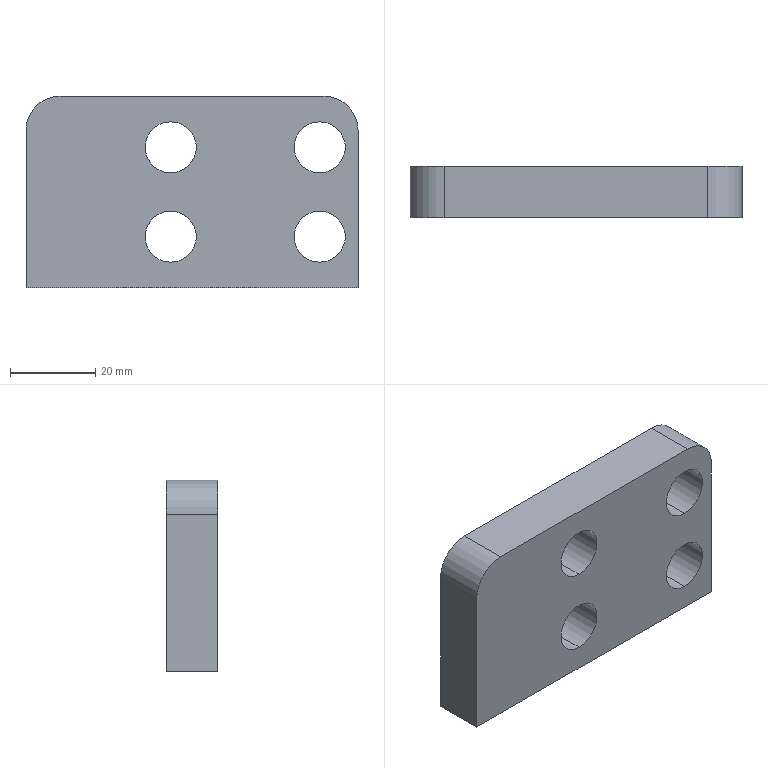Part | SolidWorks | features BaseBody 1 | 1 solid | 28 faces | box 78 x 12 x 45 mm | volume 32787 mm3 | cylinder 14 | cone 8 | plane 6 | commonest cylinder face diameters 12 x8 8.5 x4 16 x2
STEP:
#1=CARTESIAN_POINT('',(30.,0.,-16.5));
#2=VERTEX_POINT('',#1);
#3=CARTESIAN_POINT('',(30.,0.,-4.5));
#4=VERTEX_POINT('',#3);
#5=CARTESIAN_POINT('',(30.,0.,-10.5));
#6=DIRECTION('',(0.,1.,0.));
#7=DIRECTION('',(0.,0.,1.));
#8=AXIS2_PLACEMENT_3D('',#5,#6,#7);
#9=CIRCLE('',#8,6.);
#10=EDGE_CURVE('',#2,#4,#9,.T.);
#11=ORIENTED_EDGE('',*,*,#10,.F.);
#12=CARTESIAN_POINT('',(30.,12.,-16.5));
#13=VERTEX_POINT('',#12);
#14=CARTESIAN_POINT('',(30.,12.,-16.5));
#15=DIRECTION('',(0.,1.,0.));
#16=VECTOR('',#15,1000.);
#17=LINE('',#14,#16);
#18=EDGE_CURVE('',#2,#13,#17,.T.);
#19=ORIENTED_EDGE('',*,*,#18,.T.);
#20=CARTESIAN_POINT('',(30.,12.,-4.5));
#21=VERTEX_POINT('',#20);
#22=CARTESIAN_POINT('',(30.,12.,-10.5));
#23=DIRECTION('',(0.,1.,0.));
#24=DIRECTION('',(0.,0.,1.));
#25=AXIS2_PLACEMENT_3D('',#22,#23,#24);
#26=CIRCLE('',#25,6.);
#27=EDGE_CURVE('',#13,#21,#26,.T.);
#28=ORIENTED_EDGE('',*,*,#27,.T.);
#29=CARTESIAN_POINT('',(30.,12.,-4.5));
#30=DIRECTION('',(0.,1.,0.));
#31=VECTOR('',#30,1000.);
#32=LINE('',#29,#31);
#33=EDGE_CURVE('',#4,#21,#32,.T.);
#34=ORIENTED_EDGE('',*,*,#33,.F.);
#35=EDGE_LOOP('',(#11,#19,#28,#34));
#36=FACE_OUTER_BOUND('',#35,.T.);
#37=CARTESIAN_POINT('',(30.,12.,-10.5));
#38=DIRECTION('',(0.,1.,0.));
#39=DIRECTION('',(0.,0.,1.));
#40=AXIS2_PLACEMENT_3D('',#37,#38,#39);
#41=CYLINDRICAL_SURFACE('',#40,6.);
#42=ADVANCED_FACE('',(#36),#41,.F.);
#43=CARTESIAN_POINT('',(-5.,0.,-16.5));
#44=VERTEX_POINT('',#43);
#45=CARTESIAN_POINT('',(-5.,0.,-4.5));
#46=VERTEX_POINT('',#45);
#47=CARTESIAN_POINT('',(-5.,0.,-10.5));
#48=DIRECTION('',(0.,1.,0.));
#49=DIRECTION('',(0.,0.,1.));
#50=AXIS2_PLACEMENT_3D('',#47,#48,#49);
#51=CIRCLE('',#50,6.);
#52=EDGE_CURVE('',#44,#46,#51,.T.);
#53=ORIENTED_EDGE('',*,*,#52,.F.);
#54=CARTESIAN_POINT('',(-5.,12.,-16.5));
#55=VERTEX_POINT('',#54);
#56=CARTESIAN_POINT('',(-5.,12.,-16.5));
#57=DIRECTION('',(0.,1.,0.));
#58=VECTOR('',#57,1000.);
#59=LINE('',#56,#58);
#60=EDGE_CURVE('',#44,#55,#59,.T.);
#61=ORIENTED_EDGE('',*,*,#60,.T.);
#62=CARTESIAN_POINT('',(-5.,12.,-4.5));
#63=VERTEX_POINT('',#62);
#64=CARTESIAN_POINT('',(-5.,12.,-10.5));
#65=DIRECTION('',(0.,1.,0.));
#66=DIRECTION('',(0.,0.,1.));
#67=AXIS2_PLACEMENT_3D('',#64,#65,#66);
#68=CIRCLE('',#67,6.);
#69=EDGE_CURVE('',#55,#63,#68,.T.);
#70=ORIENTED_EDGE('',*,*,#69,.T.);
#71=CARTESIAN_POINT('',(-5.,12.,-4.5));
#72=DIRECTION('',(0.,1.,0.));
#73=VECTOR('',#72,1000.);
#74=LINE('',#71,#73);
#75=EDGE_CURVE('',#46,#63,#74,.T.);
#76=ORIENTED_EDGE('',*,*,#75,.F.);
#77=EDGE_LOOP('',(#53,#61,#70,#76));
#78=FACE_OUTER_BOUND('',#77,.T.);
#79=CARTESIAN_POINT('',(-5.,12.,-10.5));
#80=DIRECTION('',(0.,1.,0.));
#81=DIRECTION('',(0.,0.,1.));
#82=AXIS2_PLACEMENT_3D('',#79,#80,#81);
#83=CYLINDRICAL_SURFACE('',#82,6.);
#84=ADVANCED_FACE('',(#78),#83,.F.);
#85=CARTESIAN_POINT('',(-5.,0.,4.5));
#86=VERTEX_POINT('',#85);
#87=CARTESIAN_POINT('',(-5.,0.,16.5));
#88=VERTEX_POINT('',#87);
#89=CARTESIAN_POINT('',(-5.,0.,10.5));
#90=DIRECTION('',(0.,1.,0.));
#91=DIRECTION('',(0.,0.,1.));
#92=AXIS2_PLACEMENT_3D('',#89,#90,#91);
#93=CIRCLE('',#92,6.);
#94=EDGE_CURVE('',#86,#88,#93,.T.);
#95=ORIENTED_EDGE('',*,*,#94,.F.);
#96=CARTESIAN_POINT('',(-5.,12.,4.5));
#97=VERTEX_POINT('',#96);
#98=CARTESIAN_POINT('',(-5.,12.,4.5));
#99=DIRECTION('',(0.,1.,0.));
#100=VECTOR('',#99,1000.);
#101=LINE('',#98,#100);
#102=EDGE_CURVE('',#86,#97,#101,.T.);
#103=ORIENTED_EDGE('',*,*,#102,.T.);
#104=CARTESIAN_POINT('',(-5.,12.,16.5));
#105=VERTEX_POINT('',#104);
#106=CARTESIAN_POINT('',(-5.,12.,10.5));
#107=DIRECTION('',(0.,1.,0.));
#108=DIRECTION('',(0.,0.,1.));
#109=AXIS2_PLACEMENT_3D('',#106,#107,#108);
#110=CIRCLE('',#109,6.);
#111=EDGE_CURVE('',#97,#105,#110,.T.);
#112=ORIENTED_EDGE('',*,*,#111,.T.);
#113=CARTESIAN_POINT('',(-5.,12.,16.5));
#114=DIRECTION('',(0.,1.,0.));
#115=VECTOR('',#114,1000.);
#116=LINE('',#113,#115);
#117=EDGE_CURVE('',#88,#105,#116,.T.);
#118=ORIENTED_EDGE('',*,*,#117,.F.);
#119=EDGE_LOOP('',(#95,#103,#112,#118));
#120=FACE_OUTER_BOUND('',#119,.T.);
#121=CARTESIAN_POINT('',(-5.,12.,10.5));
#122=DIRECTION('',(0.,1.,0.));
#123=DIRECTION('',(0.,0.,1.));
#124=AXIS2_PLACEMENT_3D('',#121,#122,#123);
#125=CYLINDRICAL_SURFACE('',#124,6.);
#126=ADVANCED_FACE('',(#120),#125,.F.);
#127=CARTESIAN_POINT('',(30.,0.,4.5));
#128=VERTEX_POINT('',#127);
#129=CARTESIAN_POINT('',(30.,0.,16.5));
#130=VERTEX_POINT('',#129);
#131=CARTESIAN_POINT('',(30.,0.,10.5));
#132=DIRECTION('',(0.,1.,0.));
#133=DIRECTION('',(0.,0.,1.));
#134=AXIS2_PLACEMENT_3D('',#131,#132,#133);
#135=CIRCLE('',#134,6.);
#136=EDGE_CURVE('',#128,#130,#135,.T.);
#137=ORIENTED_EDGE('',*,*,#136,.F.);
#138=CARTESIAN_POINT('',(30.,12.,4.5));
#139=VERTEX_POINT('',#138);
#140=CARTESIAN_POINT('',(30.,12.,4.5));
#141=DIRECTION('',(0.,1.,0.));
#142=VECTOR('',#141,1000.);
#143=LINE('',#140,#142);
#144=EDGE_CURVE('',#128,#139,#143,.T.);
#145=ORIENTED_EDGE('',*,*,#144,.T.);
#146=CARTESIAN_POINT('',(30.,12.,16.5));
#147=VERTEX_POINT('',#146);
#148=CARTESIAN_POINT('',(30.,12.,10.5));
#149=DIRECTION('',(0.,1.,0.));
#150=DIRECTION('',(0.,0.,1.));
#151=AXIS2_PLACEMENT_3D('',#148,#149,#150);
#152=CIRCLE('',#151,6.);
#153=EDGE_CURVE('',#139,#147,#152,.T.);
#154=ORIENTED_EDGE('',*,*,#153,.T.);
#155=CARTESIAN_POINT('',(30.,12.,16.5));
#156=DIRECTION('',(0.,1.,0.));
#157=VECTOR('',#156,1000.);
#158=LINE('',#155,#157);
#159=EDGE_CURVE('',#130,#147,#158,.T.);
#160=ORIENTED_EDGE('',*,*,#159,.F.);
#161=EDGE_LOOP('',(#137,#145,#154,#160));
#162=FACE_OUTER_BOUND('',#161,.T.);
#163=CARTESIAN_POINT('',(30.,12.,10.5));
#164=DIRECTION('',(0.,1.,0.));
#165=DIRECTION('',(0.,0.,1.));
#166=AXIS2_PLACEMENT_3D('',#163,#164,#165);
#167=CYLINDRICAL_SURFACE('',#166,6.);
#168=ADVANCED_FACE('',(#162),#167,.F.);
#169=CARTESIAN_POINT('',(-22.75,6.,-21.725));
#170=VERTEX_POINT('',#169);
#171=CARTESIAN_POINT('',(-31.25,6.,-21.725));
#172=VERTEX_POINT('',#171);
#173=CARTESIAN_POINT('',(-27.,6.,-21.725));
#174=DIRECTION('',(0.,0.,-1.));
#175=DIRECTION('',(-1.,0.,0.));
#176=AXIS2_PLACEMENT_3D('',#173,#174,#175);
#177=CIRCLE('',#176,4.25);
#178=EDGE_CURVE('',#170,#172,#177,.T.);
#179=ORIENTED_EDGE('',*,*,#178,.F.);
#180=CARTESIAN_POINT('',(-21.975,6.,-22.5));
#181=VERTEX_POINT('',#180);
#182=CARTESIAN_POINT('',(-21.975,6.,-22.5));
#183=DIRECTION('',(0.7071,0.,-0.7071));
#184=VECTOR('',#183,1000.);
#185=LINE('',#182,#184);
#186=EDGE_CURVE('',#170,#181,#185,.T.);
#187=ORIENTED_EDGE('',*,*,#186,.T.);
#188=CARTESIAN_POINT('',(-32.025,6.,-22.5));
#189=VERTEX_POINT('',#188);
#190=CARTESIAN_POINT('',(-27.,6.,-22.5));
#191=DIRECTION('',(0.,0.,-1.));
#192=DIRECTION('',(-1.,0.,0.));
#193=AXIS2_PLACEMENT_3D('',#190,#191,#192);
#194=CIRCLE('',#193,5.025);
#195=EDGE_CURVE('',#181,#189,#194,.T.);
#196=ORIENTED_EDGE('',*,*,#195,.T.);
#197=CARTESIAN_POINT('',(-32.025,6.,-22.5));
#198=DIRECTION('',(-0.7071,0.,-0.7071));
#199=VECTOR('',#198,1000.);
#200=LINE('',#197,#199);
#201=EDGE_CURVE('',#172,#189,#200,.T.);
#202=ORIENTED_EDGE('',*,*,#201,.F.);
#203=EDGE_LOOP('',(#179,#187,#196,#202));
#204=FACE_OUTER_BOUND('',#203,.T.);
#205=CARTESIAN_POINT('',(-27.,6.,-22.5));
#206=DIRECTION('',(0.,0.,-1.));
#207=DIRECTION('',(-1.,0.,0.));
#208=AXIS2_PLACEMENT_3D('',#205,#206,#207);
#209=CONICAL_SURFACE('',#208,5.025,0.7854);
#210=ADVANCED_FACE('',(#204),#209,.F.);
#211=CARTESIAN_POINT('',(-22.75,6.,8.));
#212=VERTEX_POINT('',#211);
#213=CARTESIAN_POINT('',(-31.25,6.,8.));
#214=VERTEX_POINT('',#213);
#215=CARTESIAN_POINT('',(-27.,6.,8.));
#216=DIRECTION('',(0.,0.,-1.));
#217=DIRECTION('',(-1.,0.,0.));
#218=AXIS2_PLACEMENT_3D('',#215,#216,#217);
#219=CIRCLE('',#218,4.25);
#220=EDGE_CURVE('',#212,#214,#219,.T.);
#221=ORIENTED_EDGE('',*,*,#220,.F.);
#222=CARTESIAN_POINT('',(-22.75,6.,-22.5));
#223=DIRECTION('',(0.,0.,-1.));
#224=VECTOR('',#223,1000.);
#225=LINE('',#222,#224);
#226=EDGE_CURVE('',#212,#170,#225,.T.);
#227=ORIENTED_EDGE('',*,*,#226,.T.);
#228=ORIENTED_EDGE('',*,*,#178,.T.);
#229=CARTESIAN_POINT('',(-31.25,6.,-22.5));
#230=DIRECTION('',(0.,0.,-1.));
#231=VECTOR('',#230,1000.);
#232=LINE('',#229,#231);
#233=EDGE_CURVE('',#214,#172,#232,.T.);
#234=ORIENTED_EDGE('',*,*,#233,.F.);
#235=EDGE_LOOP('',(#221,#227,#228,#234));
#236=FACE_OUTER_BOUND('',#235,.T.);
#237=CARTESIAN_POINT('',(-27.,6.,-22.5));
#238=DIRECTION('',(0.,0.,-1.));
#239=DIRECTION('',(-1.,0.,0.));
#240=AXIS2_PLACEMENT_3D('',#237,#238,#239);
#241=CYLINDRICAL_SURFACE('',#240,4.25);
#242=ADVANCED_FACE('',(#236),#241,.F.);
#243=CARTESIAN_POINT('',(-27.,6.,10.554));
#244=VERTEX_POINT('',#243);
#245=CARTESIAN_POINT('',(-31.25,6.,8.));
#246=DIRECTION('',(-0.8572,0.,-0.515));
#247=VECTOR('',#246,1000.);
#248=LINE('',#245,#247);
#249=EDGE_CURVE('',#244,#214,#248,.T.);
#250=ORIENTED_EDGE('',*,*,#249,.F.);
#251=CARTESIAN_POINT('',(-22.75,6.,8.));
#252=DIRECTION('',(0.8572,0.,-0.515));
#253=VECTOR('',#252,1000.);
#254=LINE('',#251,#253);
#255=EDGE_CURVE('',#244,#212,#254,.T.);
#256=ORIENTED_EDGE('',*,*,#255,.T.);
#257=ORIENTED_EDGE('',*,*,#220,.T.);
#258=EDGE_LOOP('',(#250,#256,#257));
#259=FACE_OUTER_BOUND('',#258,.T.);
#260=CARTESIAN_POINT('',(-27.,6.,8.));
#261=DIRECTION('',(0.,0.,-1.));
#262=DIRECTION('',(-1.,0.,0.));
#263=AXIS2_PLACEMENT_3D('',#260,#261,#262);
#264=CONICAL_SURFACE('',#263,4.25,1.03);
#265=ADVANCED_FACE('',(#259),#264,.F.);
#266=CARTESIAN_POINT('',(21.25,6.,-21.725));
#267=VERTEX_POINT('',#266);
#268=CARTESIAN_POINT('',(12.75,6.,-21.725));
#269=VERTEX_POINT('',#268);
#270=CARTESIAN_POINT('',(17.,6.,-21.725));
#271=DIRECTION('',(0.,0.,-1.));
#272=DIRECTION('',(-1.,0.,0.));
#273=AXIS2_PLACEMENT_3D('',#270,#271,#272);
#274=CIRCLE('',#273,4.25);
#275=EDGE_CURVE('',#267,#269,#274,.T.);
#276=ORIENTED_EDGE('',*,*,#275,.F.);
#277=CARTESIAN_POINT('',(22.025,6.,-22.5));
#278=VERTEX_POINT('',#277);
#279=CARTESIAN_POINT('',(22.025,6.,-22.5));
#280=DIRECTION('',(0.7071,0.,-0.7071));
#281=VECTOR('',#280,1000.);
#282=LINE('',#279,#281);
#283=EDGE_CURVE('',#267,#278,#282,.T.);
#284=ORIENTED_EDGE('',*,*,#283,.T.);
#285=CARTESIAN_POINT('',(11.975,6.,-22.5));
#286=VERTEX_POINT('',#285);
#287=CARTESIAN_POINT('',(17.,6.,-22.5));
#288=DIRECTION('',(0.,0.,-1.));
#289=DIRECTION('',(-1.,0.,0.));
#290=AXIS2_PLACEMENT_3D('',#287,#288,#289);
#291=CIRCLE('',#290,5.025);
#292=EDGE_CURVE('',#278,#286,#291,.T.);
#293=ORIENTED_EDGE('',*,*,#292,.T.);
#294=CARTESIAN_POINT('',(11.975,6.,-22.5));
#295=DIRECTION('',(-0.7071,0.,-0.7071));
#296=VECTOR('',#295,1000.);
#297=LINE('',#294,#296);
#298=EDGE_CURVE('',#269,#286,#297,.T.);
#299=ORIENTED_EDGE('',*,*,#298,.F.);
#300=EDGE_LOOP('',(#276,#284,#293,#299));
#301=FACE_OUTER_BOUND('',#300,.T.);
#302=CARTESIAN_POINT('',(17.,6.,-22.5));
#303=DIRECTION('',(0.,0.,-1.));
#304=DIRECTION('',(-1.,0.,0.));
#305=AXIS2_PLACEMENT_3D('',#302,#303,#304);
#306=CONICAL_SURFACE('',#305,5.025,0.7854);
#307=ADVANCED_FACE('',(#301),#306,.F.);
#308=CARTESIAN_POINT('',(21.25,6.,8.));
#309=VERTEX_POINT('',#308);
#310=CARTESIAN_POINT('',(12.75,6.,8.));
#311=VERTEX_POINT('',#310);
#312=CARTESIAN_POINT('',(17.,6.,8.));
#313=DIRECTION('',(0.,0.,-1.));
#314=DIRECTION('',(-1.,0.,0.));
#315=AXIS2_PLACEMENT_3D('',#312,#313,#314);
#316=CIRCLE('',#315,4.25);
#317=EDGE_CURVE('',#309,#311,#316,.T.);
#318=ORIENTED_EDGE('',*,*,#317,.F.);
#319=CARTESIAN_POINT('',(21.25,6.,-22.5));
#320=DIRECTION('',(0.,0.,-1.));
#321=VECTOR('',#320,1000.);
#322=LINE('',#319,#321);
#323=EDGE_CURVE('',#309,#267,#322,.T.);
#324=ORIENTED_EDGE('',*,*,#323,.T.);
#325=ORIENTED_EDGE('',*,*,#275,.T.);
#326=CARTESIAN_POINT('',(12.75,6.,-22.5));
#327=DIRECTION('',(0.,0.,-1.));
#328=VECTOR('',#327,1000.);
#329=LINE('',#326,#328);
#330=EDGE_CURVE('',#311,#269,#329,.T.);
#331=ORIENTED_EDGE('',*,*,#330,.F.);
#332=EDGE_LOOP('',(#318,#324,#325,#331));
#333=FACE_OUTER_BOUND('',#332,.T.);
#334=CARTESIAN_POINT('',(17.,6.,-22.5));
#335=DIRECTION('',(0.,0.,-1.));
#336=DIRECTION('',(-1.,0.,0.));
#337=AXIS2_PLACEMENT_3D('',#334,#335,#336);
#338=CYLINDRICAL_SURFACE('',#337,4.25);
#339=ADVANCED_FACE('',(#333),#338,.F.);
#340=CARTESIAN_POINT('',(17.,6.,10.554));
#341=VERTEX_POINT('',#340);
#342=CARTESIAN_POINT('',(12.75,6.,8.));
#343=DIRECTION('',(-0.8572,0.,-0.515));
#344=VECTOR('',#343,1000.);
#345=LINE('',#342,#344);
#346=EDGE_CURVE('',#341,#311,#345,.T.);
#347=ORIENTED_EDGE('',*,*,#346,.F.);
#348=CARTESIAN_POINT('',(21.25,6.,8.));
#349=DIRECTION('',(0.8572,0.,-0.515));
#350=VECTOR('',#349,1000.);
#351=LINE('',#348,#350);
#352=EDGE_CURVE('',#341,#309,#351,.T.);
#353=ORIENTED_EDGE('',*,*,#352,.T.);
#354=ORIENTED_EDGE('',*,*,#317,.T.);
#355=EDGE_LOOP('',(#347,#353,#354));
#356=FACE_OUTER_BOUND('',#355,.T.);
#357=CARTESIAN_POINT('',(17.,6.,8.));
#358=DIRECTION('',(0.,0.,-1.));
#359=DIRECTION('',(-1.,0.,0.));
#360=AXIS2_PLACEMENT_3D('',#357,#358,#359);
#361=CONICAL_SURFACE('',#360,4.25,1.03);
#362=ADVANCED_FACE('',(#356),#361,.F.);
#363=CARTESIAN_POINT('',(39.,12.,14.5));
#364=VERTEX_POINT('',#363);
#365=CARTESIAN_POINT('',(39.,12.,-22.5));
#366=VERTEX_POINT('',#365);
#367=CARTESIAN_POINT('',(39.,12.,-22.5));
#368=DIRECTION('',(0.,0.,-1.));
#369=VECTOR('',#368,1000.);
#370=LINE('',#367,#369);
#371=EDGE_CURVE('',#364,#366,#370,.T.);
#372=ORIENTED_EDGE('',*,*,#371,.F.);
#373=CARTESIAN_POINT('',(39.,0.,14.5));
#374=VERTEX_POINT('',#373);
#375=CARTESIAN_POINT('',(39.,12.,14.5));
#376=DIRECTION('',(0.,-1.,0.));
#377=VECTOR('',#376,1000.);
#378=LINE('',#375,#377);
#379=EDGE_CURVE('',#364,#374,#378,.T.);
#380=ORIENTED_EDGE('',*,*,#379,.T.);
#381=CARTESIAN_POINT('',(39.,0.,-22.5));
#382=VERTEX_POINT('',#381);
#383=CARTESIAN_POINT('',(39.,0.,-22.5));
#384=DIRECTION('',(0.,0.,-1.));
#385=VECTOR('',#384,1000.);
#386=LINE('',#383,#385);
#387=EDGE_CURVE('',#374,#382,#386,.T.);
#388=ORIENTED_EDGE('',*,*,#387,.T.);
#389=CARTESIAN_POINT('',(39.,12.,-22.5));
#390=DIRECTION('',(0.,-1.,0.));
#391=VECTOR('',#390,1000.);
#392=LINE('',#389,#391);
#393=EDGE_CURVE('',#366,#382,#392,.T.);
#394=ORIENTED_EDGE('',*,*,#393,.F.);
#395=EDGE_LOOP('',(#372,#380,#388,#394));
#396=FACE_OUTER_BOUND('',#395,.T.);
#397=CARTESIAN_POINT('',(39.,12.,-22.5));
#398=DIRECTION('',(-1.,0.,0.));
#399=DIRECTION('',(0.,0.,1.));
#400=AXIS2_PLACEMENT_3D('',#397,#398,#399);
#401=PLANE('',#400);
#402=ADVANCED_FACE('',(#396),#401,.F.);
#403=CARTESIAN_POINT('',(-27.,6.,-22.5));
#404=DIRECTION('',(0.,0.,-1.));
#405=DIRECTION('',(-1.,0.,0.));
#406=AXIS2_PLACEMENT_3D('',#403,#404,#405);
#407=CIRCLE('',#406,5.025);
#408=EDGE_CURVE('',#189,#181,#407,.T.);
#409=ORIENTED_EDGE('',*,*,#408,.F.);
#410=ORIENTED_EDGE('',*,*,#195,.F.);
#411=EDGE_LOOP('',(#409,#410));
#412=FACE_BOUND('',#411,.T.);
#413=CARTESIAN_POINT('',(17.,6.,-22.5));
#414=DIRECTION('',(0.,0.,-1.));
#415=DIRECTION('',(-1.,0.,0.));
#416=AXIS2_PLACEMENT_3D('',#413,#414,#415);
#417=CIRCLE('',#416,5.025);
#418=EDGE_CURVE('',#286,#278,#417,.T.);
#419=ORIENTED_EDGE('',*,*,#418,.F.);
#420=ORIENTED_EDGE('',*,*,#292,.F.);
#421=EDGE_LOOP('',(#419,#420));
#422=FACE_BOUND('',#421,.T.);
#423=CARTESIAN_POINT('',(-39.,0.,-22.5));
#424=VERTEX_POINT('',#423);
#425=CARTESIAN_POINT('',(-39.,0.,-22.5));
#426=DIRECTION('',(-1.,0.,0.));
#427=VECTOR('',#426,1000.);
#428=LINE('',#425,#427);
#429=EDGE_CURVE('',#382,#424,#428,.T.);
#430=ORIENTED_EDGE('',*,*,#429,.T.);
#431=CARTESIAN_POINT('',(-39.,12.,-22.5));
#432=VERTEX_POINT('',#431);
#433=CARTESIAN_POINT('',(-39.,12.,-22.5));
#434=DIRECTION('',(0.,-1.,0.));
#435=VECTOR('',#434,1000.);
#436=LINE('',#433,#435);
#437=EDGE_CURVE('',#432,#424,#436,.T.);
#438=ORIENTED_EDGE('',*,*,#437,.F.);
#439=CARTESIAN_POINT('',(-39.,12.,-22.5));
#440=DIRECTION('',(-1.,0.,0.));
#441=VECTOR('',#440,1000.);
#442=LINE('',#439,#441);
#443=EDGE_CURVE('',#366,#432,#442,.T.);
#444=ORIENTED_EDGE('',*,*,#443,.F.);
#445=ORIENTED_EDGE('',*,*,#393,.T.);
#446=EDGE_LOOP('',(#430,#438,#444,#445));
#447=FACE_OUTER_BOUND('',#446,.T.);
#448=CARTESIAN_POINT('',(-39.,12.,-22.5));
#449=DIRECTION('',(0.,0.,1.));
#450=DIRECTION('',(1.,0.,0.));
#451=AXIS2_PLACEMENT_3D('',#448,#449,#450);
#452=PLANE('',#451);
#453=ADVANCED_FACE('',(#412,#422,#447),#452,.F.);
#454=CARTESIAN_POINT('',(-39.,0.,14.5));
#455=VERTEX_POINT('',#454);
#456=CARTESIAN_POINT('',(-39.,0.,-22.5));
#457=DIRECTION('',(0.,0.,1.));
#458=VECTOR('',#457,1000.);
#459=LINE('',#456,#458);
#460=EDGE_CURVE('',#424,#455,#459,.T.);
#461=ORIENTED_EDGE('',*,*,#460,.T.);
#462=CARTESIAN_POINT('',(-39.,12.,14.5));
#463=VERTEX_POINT('',#462);
#464=CARTESIAN_POINT('',(-39.,12.,14.5));
#465=DIRECTION('',(0.,1.,0.));
#466=VECTOR('',#465,1000.);
#467=LINE('',#464,#466);
#468=EDGE_CURVE('',#455,#463,#467,.T.);
#469=ORIENTED_EDGE('',*,*,#468,.T.);
#470=CARTESIAN_POINT('',(-39.,12.,-22.5));
#471=DIRECTION('',(0.,0.,1.));
#472=VECTOR('',#471,1000.);
#473=LINE('',#470,#472);
#474=EDGE_CURVE('',#432,#463,#473,.T.);
#475=ORIENTED_EDGE('',*,*,#474,.F.);
#476=ORIENTED_EDGE('',*,*,#437,.T.);
#477=EDGE_LOOP('',(#461,#469,#475,#476));
#478=FACE_OUTER_BOUND('',#477,.T.);
#479=CARTESIAN_POINT('',(-39.,12.,-22.5));
#480=DIRECTION('',(1.,0.,0.));
#481=DIRECTION('',(0.,0.,-1.));
#482=AXIS2_PLACEMENT_3D('',#479,#480,#481);
#483=PLANE('',#482);
#484=ADVANCED_FACE('',(#478),#483,.F.);
#485=CARTESIAN_POINT('',(-31.,0.,22.5));
#486=VERTEX_POINT('',#485);
#487=CARTESIAN_POINT('',(31.,0.,22.5));
#488=VERTEX_POINT('',#487);
#489=CARTESIAN_POINT('',(-39.,0.,22.5));
#490=DIRECTION('',(1.,0.,0.));
#491=VECTOR('',#490,1000.);
#492=LINE('',#489,#491);
#493=EDGE_CURVE('',#486,#488,#492,.T.);
#494=ORIENTED_EDGE('',*,*,#493,.T.);
#495=CARTESIAN_POINT('',(31.,12.,22.5));
#496=VERTEX_POINT('',#495);
#497=CARTESIAN_POINT('',(31.,12.,22.5));
#498=DIRECTION('',(0.,1.,0.));
#499=VECTOR('',#498,1000.);
#500=LINE('',#497,#499);
#501=EDGE_CURVE('',#488,#496,#500,.T.);
#502=ORIENTED_EDGE('',*,*,#501,.T.);
#503=CARTESIAN_POINT('',(-31.,12.,22.5));
#504=VERTEX_POINT('',#503);
#505=CARTESIAN_POINT('',(-39.,12.,22.5));
#506=DIRECTION('',(1.,0.,0.));
#507=VECTOR('',#506,1000.);
#508=LINE('',#505,#507);
#509=EDGE_CURVE('',#504,#496,#508,.T.);
#510=ORIENTED_EDGE('',*,*,#509,.F.);
#511=CARTESIAN_POINT('',(-31.,12.,22.5));
#512=DIRECTION('',(0.,-1.,0.));
#513=VECTOR('',#512,1000.);
#514=LINE('',#511,#513);
#515=EDGE_CURVE('',#504,#486,#514,.T.);
#516=ORIENTED_EDGE('',*,*,#515,.T.);
#517=EDGE_LOOP('',(#494,#502,#510,#516));
#518=FACE_OUTER_BOUND('',#517,.T.);
#519=CARTESIAN_POINT('',(-39.,12.,22.5));
#520=DIRECTION('',(0.,0.,-1.));
#521=DIRECTION('',(-1.,0.,0.));
#522=AXIS2_PLACEMENT_3D('',#519,#520,#521);
#523=PLANE('',#522);
#524=ADVANCED_FACE('',(#518),#523,.F.);
#525=CARTESIAN_POINT('',(30.,12.,-10.5));
#526=DIRECTION('',(0.,1.,0.));
#527=DIRECTION('',(0.,0.,1.));
#528=AXIS2_PLACEMENT_3D('',#525,#526,#527);
#529=CIRCLE('',#528,6.);
#530=EDGE_CURVE('',#21,#13,#529,.T.);
#531=ORIENTED_EDGE('',*,*,#530,.F.);
#532=ORIENTED_EDGE('',*,*,#27,.F.);
#533=EDGE_LOOP('',(#531,#532));
#534=FACE_BOUND('',#533,.T.);
#535=CARTESIAN_POINT('',(-5.,12.,-10.5));
#536=DIRECTION('',(0.,1.,0.));
#537=DIRECTION('',(0.,0.,1.));
#538=AXIS2_PLACEMENT_3D('',#535,#536,#537);
#539=CIRCLE('',#538,6.);
#540=EDGE_CURVE('',#63,#55,#539,.T.);
#541=ORIENTED_EDGE('',*,*,#540,.F.);
#542=ORIENTED_EDGE('',*,*,#69,.F.);
#543=EDGE_LOOP('',(#541,#542));
#544=FACE_BOUND('',#543,.T.);
#545=CARTESIAN_POINT('',(-5.,12.,10.5));
#546=DIRECTION('',(0.,1.,0.));
#547=DIRECTION('',(0.,0.,1.));
#548=AXIS2_PLACEMENT_3D('',#545,#546,#547);
#549=CIRCLE('',#548,6.);
#550=EDGE_CURVE('',#105,#97,#549,.T.);
#551=ORIENTED_EDGE('',*,*,#550,.F.);
#552=ORIENTED_EDGE('',*,*,#111,.F.);
#553=EDGE_LOOP('',(#551,#552));
#554=FACE_BOUND('',#553,.T.);
#555=CARTESIAN_POINT('',(30.,12.,10.5));
#556=DIRECTION('',(0.,1.,0.));
#557=DIRECTION('',(0.,0.,1.));
#558=AXIS2_PLACEMENT_3D('',#555,#556,#557);
#559=CIRCLE('',#558,6.);
#560=EDGE_CURVE('',#147,#139,#559,.T.);
#561=ORIENTED_EDGE('',*,*,#560,.F.);
#562=ORIENTED_EDGE('',*,*,#153,.F.);
#563=EDGE_LOOP('',(#561,#562));
#564=FACE_BOUND('',#563,.T.);
#565=ORIENTED_EDGE('',*,*,#509,.T.);
#566=CARTESIAN_POINT('',(31.,12.,14.5));
#567=DIRECTION('',(0.,1.,0.));
#568=DIRECTION('',(0.,0.,1.));
#569=AXIS2_PLACEMENT_3D('',#566,#567,#568);
#570=CIRCLE('',#569,8.);
#571=EDGE_CURVE('',#496,#364,#570,.T.);
#572=ORIENTED_EDGE('',*,*,#571,.T.);
#573=ORIENTED_EDGE('',*,*,#371,.T.);
#574=ORIENTED_EDGE('',*,*,#443,.T.);
#575=ORIENTED_EDGE('',*,*,#474,.T.);
#576=CARTESIAN_POINT('',(-31.,12.,14.5));
#577=DIRECTION('',(0.,1.,0.));
#578=DIRECTION('',(0.,0.,1.));
#579=AXIS2_PLACEMENT_3D('',#576,#577,#578);
#580=CIRCLE('',#579,8.);
#581=EDGE_CURVE('',#463,#504,#580,.T.);
#582=ORIENTED_EDGE('',*,*,#581,.T.);
#583=EDGE_LOOP('',(#565,#572,#573,#574,#575,#582));
#584=FACE_OUTER_BOUND('',#583,.T.);
#585=CARTESIAN_POINT('',(0.,12.,0.));
#586=DIRECTION('',(0.,1.,0.));
#587=DIRECTION('',(0.,0.,1.));
#588=AXIS2_PLACEMENT_3D('',#585,#586,#587);
#589=PLANE('',#588);
#590=ADVANCED_FACE('',(#534,#544,#554,#564,#584),#589,.T.);
#591=CARTESIAN_POINT('',(30.,0.,-10.5));
#592=DIRECTION('',(0.,1.,0.));
#593=DIRECTION('',(0.,0.,1.));
#594=AXIS2_PLACEMENT_3D('',#591,#592,#593);
#595=CIRCLE('',#594,6.);
#596=EDGE_CURVE('',#4,#2,#595,.T.);
#597=ORIENTED_EDGE('',*,*,#596,.T.);
#598=ORIENTED_EDGE('',*,*,#10,.T.);
#599=EDGE_LOOP('',(#597,#598));
#600=FACE_BOUND('',#599,.T.);
#601=CARTESIAN_POINT('',(-5.,0.,-10.5));
#602=DIRECTION('',(0.,1.,0.));
#603=DIRECTION('',(0.,0.,1.));
#604=AXIS2_PLACEMENT_3D('',#601,#602,#603);
#605=CIRCLE('',#604,6.);
#606=EDGE_CURVE('',#46,#44,#605,.T.);
#607=ORIENTED_EDGE('',*,*,#606,.T.);
#608=ORIENTED_EDGE('',*,*,#52,.T.);
#609=EDGE_LOOP('',(#607,#608));
#610=FACE_BOUND('',#609,.T.);
#611=CARTESIAN_POINT('',(-5.,0.,10.5));
#612=DIRECTION('',(0.,1.,0.));
#613=DIRECTION('',(0.,0.,1.));
#614=AXIS2_PLACEMENT_3D('',#611,#612,#613);
#615=CIRCLE('',#614,6.);
#616=EDGE_CURVE('',#88,#86,#615,.T.);
#617=ORIENTED_EDGE('',*,*,#616,.T.);
#618=ORIENTED_EDGE('',*,*,#94,.T.);
#619=EDGE_LOOP('',(#617,#618));
#620=FACE_BOUND('',#619,.T.);
#621=CARTESIAN_POINT('',(30.,0.,10.5));
#622=DIRECTION('',(0.,1.,0.));
#623=DIRECTION('',(0.,0.,1.));
#624=AXIS2_PLACEMENT_3D('',#621,#622,#623);
#625=CIRCLE('',#624,6.);
#626=EDGE_CURVE('',#130,#128,#625,.T.);
#627=ORIENTED_EDGE('',*,*,#626,.T.);
#628=ORIENTED_EDGE('',*,*,#136,.T.);
#629=EDGE_LOOP('',(#627,#628));
#630=FACE_BOUND('',#629,.T.);
#631=ORIENTED_EDGE('',*,*,#387,.F.);
#632=CARTESIAN_POINT('',(31.,0.,14.5));
#633=DIRECTION('',(0.,-1.,0.));
#634=DIRECTION('',(0.,0.,1.));
#635=AXIS2_PLACEMENT_3D('',#632,#633,#634);
#636=CIRCLE('',#635,8.);
#637=EDGE_CURVE('',#374,#488,#636,.T.);
#638=ORIENTED_EDGE('',*,*,#637,.T.);
#639=ORIENTED_EDGE('',*,*,#493,.F.);
#640=CARTESIAN_POINT('',(-31.,0.,14.5));
#641=DIRECTION('',(0.,-1.,0.));
#642=DIRECTION('',(0.,0.,1.));
#643=AXIS2_PLACEMENT_3D('',#640,#641,#642);
#644=CIRCLE('',#643,8.);
#645=EDGE_CURVE('',#486,#455,#644,.T.);
#646=ORIENTED_EDGE('',*,*,#645,.T.);
#647=ORIENTED_EDGE('',*,*,#460,.F.);
#648=ORIENTED_EDGE('',*,*,#429,.F.);
#649=EDGE_LOOP('',(#631,#638,#639,#646,#647,#648));
#650=FACE_OUTER_BOUND('',#649,.T.);
#651=CARTESIAN_POINT('',(0.,0.,0.));
#652=DIRECTION('',(0.,1.,0.));
#653=DIRECTION('',(0.,0.,1.));
#654=AXIS2_PLACEMENT_3D('',#651,#652,#653);
#655=PLANE('',#654);
#656=ADVANCED_FACE('',(#600,#610,#620,#630,#650),#655,.F.);
#657=ORIENTED_EDGE('',*,*,#571,.F.);
#658=ORIENTED_EDGE('',*,*,#501,.F.);
#659=ORIENTED_EDGE('',*,*,#637,.F.);
#660=ORIENTED_EDGE('',*,*,#379,.F.);
#661=EDGE_LOOP('',(#657,#658,#659,#660));
#662=FACE_OUTER_BOUND('',#661,.T.);
#663=CARTESIAN_POINT('',(31.,12.,14.5));
#664=DIRECTION('',(0.,-1.,0.));
#665=DIRECTION('',(0.,0.,-1.));
#666=AXIS2_PLACEMENT_3D('',#663,#664,#665);
#667=CYLINDRICAL_SURFACE('',#666,8.);
#668=ADVANCED_FACE('',(#662),#667,.T.);
#669=ORIENTED_EDGE('',*,*,#581,.F.);
#670=ORIENTED_EDGE('',*,*,#468,.F.);
#671=ORIENTED_EDGE('',*,*,#645,.F.);
#672=ORIENTED_EDGE('',*,*,#515,.F.);
#673=EDGE_LOOP('',(#669,#670,#671,#672));
#674=FACE_OUTER_BOUND('',#673,.T.);
#675=CARTESIAN_POINT('',(-31.,12.,14.5));
#676=DIRECTION('',(0.,-1.,0.));
#677=DIRECTION('',(0.,0.,-1.));
#678=AXIS2_PLACEMENT_3D('',#675,#676,#677);
#679=CYLINDRICAL_SURFACE('',#678,8.);
#680=ADVANCED_FACE('',(#674),#679,.T.);
#681=ORIENTED_EDGE('',*,*,#352,.F.);
#682=ORIENTED_EDGE('',*,*,#346,.T.);
#683=CARTESIAN_POINT('',(17.,6.,8.));
#684=DIRECTION('',(0.,0.,-1.));
#685=DIRECTION('',(-1.,0.,0.));
#686=AXIS2_PLACEMENT_3D('',#683,#684,#685);
#687=CIRCLE('',#686,4.25);
#688=EDGE_CURVE('',#311,#309,#687,.T.);
#689=ORIENTED_EDGE('',*,*,#688,.T.);
#690=EDGE_LOOP('',(#681,#682,#689));
#691=FACE_OUTER_BOUND('',#690,.T.);
#692=CARTESIAN_POINT('',(17.,6.,8.));
#693=DIRECTION('',(0.,0.,-1.));
#694=DIRECTION('',(-1.,0.,0.));
#695=AXIS2_PLACEMENT_3D('',#692,#693,#694);
#696=CONICAL_SURFACE('',#695,4.25,1.03);
#697=ADVANCED_FACE('',(#691),#696,.F.);
#698=ORIENTED_EDGE('',*,*,#323,.F.);
#699=ORIENTED_EDGE('',*,*,#688,.F.);
#700=ORIENTED_EDGE('',*,*,#330,.T.);
#701=CARTESIAN_POINT('',(17.,6.,-21.725));
#702=DIRECTION('',(0.,0.,-1.));
#703=DIRECTION('',(-1.,0.,0.));
#704=AXIS2_PLACEMENT_3D('',#701,#702,#703);
#705=CIRCLE('',#704,4.25);
#706=EDGE_CURVE('',#269,#267,#705,.T.);
#707=ORIENTED_EDGE('',*,*,#706,.T.);
#708=EDGE_LOOP('',(#698,#699,#700,#707));
#709=FACE_OUTER_BOUND('',#708,.T.);
#710=CARTESIAN_POINT('',(17.,6.,-22.5));
#711=DIRECTION('',(0.,0.,-1.));
#712=DIRECTION('',(-1.,0.,0.));
#713=AXIS2_PLACEMENT_3D('',#710,#711,#712);
#714=CYLINDRICAL_SURFACE('',#713,4.25);
#715=ADVANCED_FACE('',(#709),#714,.F.);
#716=ORIENTED_EDGE('',*,*,#283,.F.);
#717=ORIENTED_EDGE('',*,*,#706,.F.);
#718=ORIENTED_EDGE('',*,*,#298,.T.);
#719=ORIENTED_EDGE('',*,*,#418,.T.);
#720=EDGE_LOOP('',(#716,#717,#718,#719));
#721=FACE_OUTER_BOUND('',#720,.T.);
#722=CARTESIAN_POINT('',(17.,6.,-22.5));
#723=DIRECTION('',(0.,0.,-1.));
#724=DIRECTION('',(-1.,0.,0.));
#725=AXIS2_PLACEMENT_3D('',#722,#723,#724);
#726=CONICAL_SURFACE('',#725,5.025,0.7854);
#727=ADVANCED_FACE('',(#721),#726,.F.);
#728=ORIENTED_EDGE('',*,*,#255,.F.);
#729=ORIENTED_EDGE('',*,*,#249,.T.);
#730=CARTESIAN_POINT('',(-27.,6.,8.));
#731=DIRECTION('',(0.,0.,-1.));
#732=DIRECTION('',(-1.,0.,0.));
#733=AXIS2_PLACEMENT_3D('',#730,#731,#732);
#734=CIRCLE('',#733,4.25);
#735=EDGE_CURVE('',#214,#212,#734,.T.);
#736=ORIENTED_EDGE('',*,*,#735,.T.);
#737=EDGE_LOOP('',(#728,#729,#736));
#738=FACE_OUTER_BOUND('',#737,.T.);
#739=CARTESIAN_POINT('',(-27.,6.,8.));
#740=DIRECTION('',(0.,0.,-1.));
#741=DIRECTION('',(-1.,0.,0.));
#742=AXIS2_PLACEMENT_3D('',#739,#740,#741);
#743=CONICAL_SURFACE('',#742,4.25,1.03);
#744=ADVANCED_FACE('',(#738),#743,.F.);
#745=ORIENTED_EDGE('',*,*,#226,.F.);
#746=ORIENTED_EDGE('',*,*,#735,.F.);
#747=ORIENTED_EDGE('',*,*,#233,.T.);
#748=CARTESIAN_POINT('',(-27.,6.,-21.725));
#749=DIRECTION('',(0.,0.,-1.));
#750=DIRECTION('',(-1.,0.,0.));
#751=AXIS2_PLACEMENT_3D('',#748,#749,#750);
#752=CIRCLE('',#751,4.25);
#753=EDGE_CURVE('',#172,#170,#752,.T.);
#754=ORIENTED_EDGE('',*,*,#753,.T.);
#755=EDGE_LOOP('',(#745,#746,#747,#754));
#756=FACE_OUTER_BOUND('',#755,.T.);
#757=CARTESIAN_POINT('',(-27.,6.,-22.5));
#758=DIRECTION('',(0.,0.,-1.));
#759=DIRECTION('',(-1.,0.,0.));
#760=AXIS2_PLACEMENT_3D('',#757,#758,#759);
#761=CYLINDRICAL_SURFACE('',#760,4.25);
#762=ADVANCED_FACE('',(#756),#761,.F.);
#763=ORIENTED_EDGE('',*,*,#186,.F.);
#764=ORIENTED_EDGE('',*,*,#753,.F.);
#765=ORIENTED_EDGE('',*,*,#201,.T.);
#766=ORIENTED_EDGE('',*,*,#408,.T.);
#767=EDGE_LOOP('',(#763,#764,#765,#766));
#768=FACE_OUTER_BOUND('',#767,.T.);
#769=CARTESIAN_POINT('',(-27.,6.,-22.5));
#770=DIRECTION('',(0.,0.,-1.));
#771=DIRECTION('',(-1.,0.,0.));
#772=AXIS2_PLACEMENT_3D('',#769,#770,#771);
#773=CONICAL_SURFACE('',#772,5.025,0.7854);
#774=ADVANCED_FACE('',(#768),#773,.F.);
#775=ORIENTED_EDGE('',*,*,#144,.F.);
#776=ORIENTED_EDGE('',*,*,#626,.F.);
#777=ORIENTED_EDGE('',*,*,#159,.T.);
#778=ORIENTED_EDGE('',*,*,#560,.T.);
#779=EDGE_LOOP('',(#775,#776,#777,#778));
#780=FACE_OUTER_BOUND('',#779,.T.);
#781=CARTESIAN_POINT('',(30.,12.,10.5));
#782=DIRECTION('',(0.,1.,0.));
#783=DIRECTION('',(0.,0.,1.));
#784=AXIS2_PLACEMENT_3D('',#781,#782,#783);
#785=CYLINDRICAL_SURFACE('',#784,6.);
#786=ADVANCED_FACE('',(#780),#785,.F.);
#787=ORIENTED_EDGE('',*,*,#102,.F.);
#788=ORIENTED_EDGE('',*,*,#616,.F.);
#789=ORIENTED_EDGE('',*,*,#117,.T.);
#790=ORIENTED_EDGE('',*,*,#550,.T.);
#791=EDGE_LOOP('',(#787,#788,#789,#790));
#792=FACE_OUTER_BOUND('',#791,.T.);
#793=CARTESIAN_POINT('',(-5.,12.,10.5));
#794=DIRECTION('',(0.,1.,0.));
#795=DIRECTION('',(0.,0.,1.));
#796=AXIS2_PLACEMENT_3D('',#793,#794,#795);
#797=CYLINDRICAL_SURFACE('',#796,6.);
#798=ADVANCED_FACE('',(#792),#797,.F.);
#799=ORIENTED_EDGE('',*,*,#60,.F.);
#800=ORIENTED_EDGE('',*,*,#606,.F.);
#801=ORIENTED_EDGE('',*,*,#75,.T.);
#802=ORIENTED_EDGE('',*,*,#540,.T.);
#803=EDGE_LOOP('',(#799,#800,#801,#802));
#804=FACE_OUTER_BOUND('',#803,.T.);
#805=CARTESIAN_POINT('',(-5.,12.,-10.5));
#806=DIRECTION('',(0.,1.,0.));
#807=DIRECTION('',(0.,0.,1.));
#808=AXIS2_PLACEMENT_3D('',#805,#806,#807);
#809=CYLINDRICAL_SURFACE('',#808,6.);
#810=ADVANCED_FACE('',(#804),#809,.F.);
#811=ORIENTED_EDGE('',*,*,#18,.F.);
#812=ORIENTED_EDGE('',*,*,#596,.F.);
#813=ORIENTED_EDGE('',*,*,#33,.T.);
#814=ORIENTED_EDGE('',*,*,#530,.T.);
#815=EDGE_LOOP('',(#811,#812,#813,#814));
#816=FACE_OUTER_BOUND('',#815,.T.);
#817=CARTESIAN_POINT('',(30.,12.,-10.5));
#818=DIRECTION('',(0.,1.,0.));
#819=DIRECTION('',(0.,0.,1.));
#820=AXIS2_PLACEMENT_3D('',#817,#818,#819);
#821=CYLINDRICAL_SURFACE('',#820,6.);
#822=ADVANCED_FACE('',(#816),#821,.F.);
#823=CLOSED_SHELL('',(#42,#84,#126,#168,#210,#242,#265,#307,#339,#362,#402,#453,#484,#524,#590,#656,#668,#680,#697,#715,#727,#744,#762,#774,#786,#798,#810,#822));
#824=MANIFOLD_SOLID_BREP('',#823);
#825=CARTESIAN_POINT('',(0.,0.,0.));
#826=DIRECTION('',(0.,0.,1.));
#827=DIRECTION('',(1.,0.,0.));
#828=AXIS2_PLACEMENT_3D('',#825,#826,#827);
#829=(LENGTH_UNIT()NAMED_UNIT(*)SI_UNIT(.MILLI.,.METRE.));
#830=UNCERTAINTY_MEASURE_WITH_UNIT(LENGTH_MEASURE(0.00001),#829,'','');
#831=(NAMED_UNIT(*)PLANE_ANGLE_UNIT()SI_UNIT($,.RADIAN.));
#832=(NAMED_UNIT(*)SI_UNIT($,.STERADIAN.)SOLID_ANGLE_UNIT());
#833=(GEOMETRIC_REPRESENTATION_CONTEXT(3)GLOBAL_UNCERTAINTY_ASSIGNED_CONTEXT((#830))GLOBAL_UNIT_ASSIGNED_CONTEXT((#829,#831,#832))REPRESENTATION_CONTEXT('',''));
#834=ADVANCED_BREP_SHAPE_REPRESENTATION('',(#824,#828),#833);